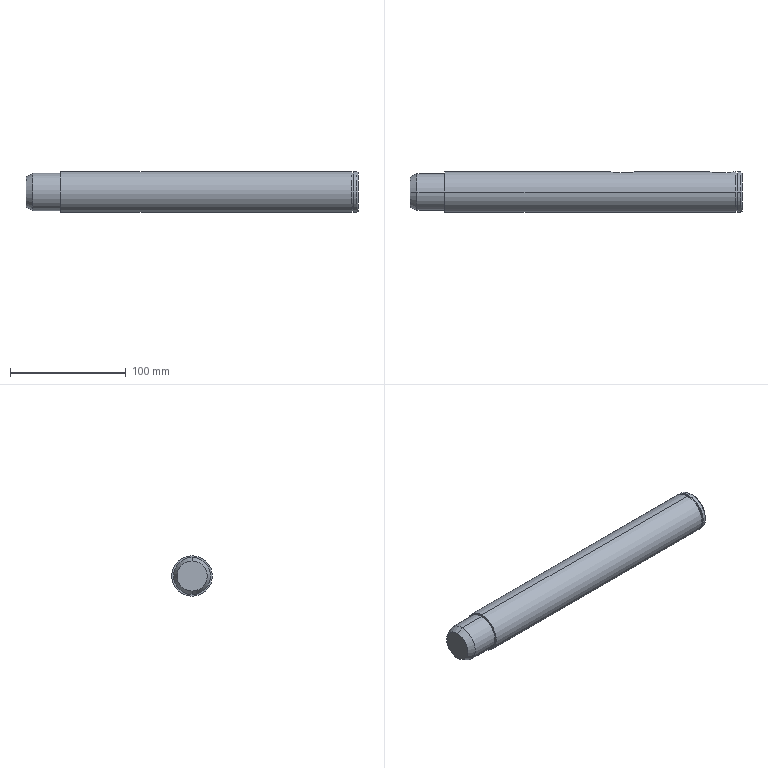Part | STEP file | 02-Support shaft 3 | 1 solid | 27 faces | box 286.5 x 35 x 35 mm | volume 267927 mm3 | cylinder 12 | plane 11 | cone 4 | commonest cylinder face diameters 10 x4 35 x4 32 x2 33 x2